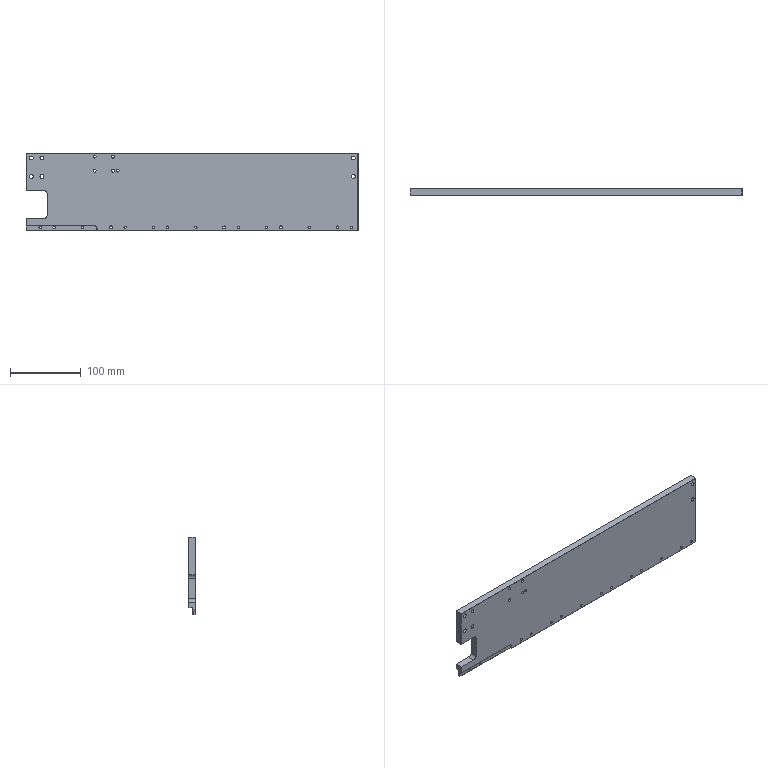Part | NX | 1 solid | 148 faces | box 469 x 10 x 110 mm | volume 472239 mm3 | cylinder 63 | cone 45 | plane 40 | commonest cylinder face diameters 3.3 x18 4 x14 5.5 x12 4.2 x8 9.5 x8 10 x2